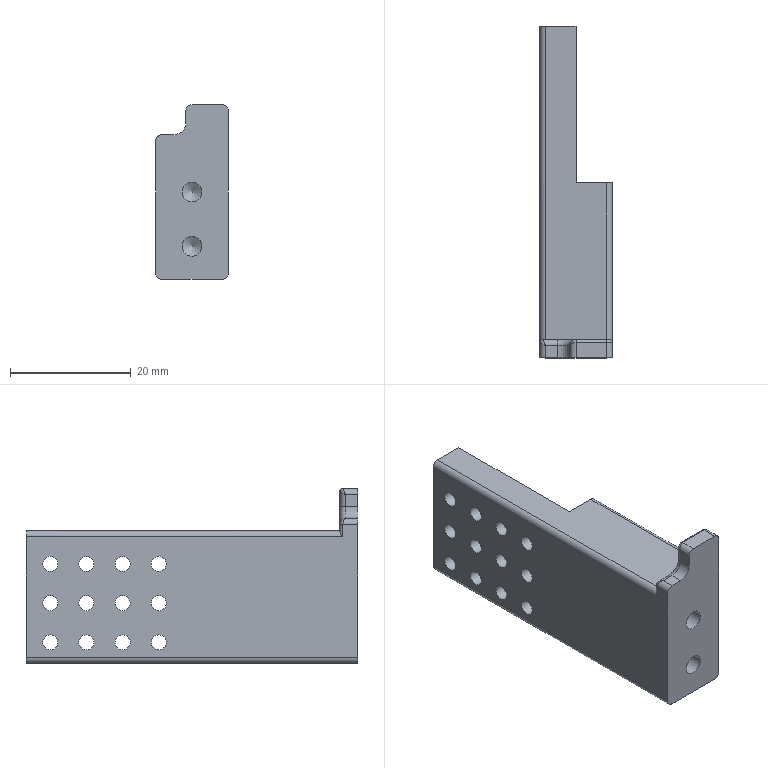Part | 1 solid | 45 faces | box 12 x 55 x 29 mm | volume 10696 mm3 | cylinder 27 | plane 12 | spline 2 | torus 2 | cone 2 | commonest cylinder face diameters 2.5 x12 2 x9 1 x3 3.3 x2 4 x1
STEP:
#1=CARTESIAN_POINT('',(12.,0.,18.));
#2=VERTEX_POINT('',#1);
#3=CARTESIAN_POINT('',(11.,0.,17.));
#4=VERTEX_POINT('',#3);
#5=CARTESIAN_POINT('',(12.,0.,17.));
#6=DIRECTION('',(0.,-1.,0.));
#7=DIRECTION('',(0.,0.,-1.));
#8=AXIS2_PLACEMENT_3D('',#5,#6,#7);
#9=CIRCLE('',#8,1.);
#10=EDGE_CURVE('',#2,#4,#9,.T.);
#11=ORIENTED_EDGE('',*,*,#10,.F.);
#12=CARTESIAN_POINT('',(12.,2.5,18.));
#13=VERTEX_POINT('',#12);
#14=CARTESIAN_POINT('',(12.,0.,18.));
#15=DIRECTION('',(0.,-1.,0.));
#16=VECTOR('',#15,1000.);
#17=LINE('',#14,#16);
#18=EDGE_CURVE('',#13,#2,#17,.T.);
#19=ORIENTED_EDGE('',*,*,#18,.F.);
#20=CARTESIAN_POINT('',(11.,2.,17.));
#21=VERTEX_POINT('',#20);
#22=CARTESIAN_POINT('',(12.,2.,17.));
#23=DIRECTION('',(0.,-0.8944,0.4472));
#24=DIRECTION('',(0.,0.4472,0.8944));
#25=AXIS2_PLACEMENT_3D('',#22,#23,#24);
#26=ELLIPSE('',#25,1.118,1.);
#27=EDGE_CURVE('',#13,#21,#26,.T.);
#28=ORIENTED_EDGE('',*,*,#27,.T.);
#29=CARTESIAN_POINT('',(11.,0.,17.));
#30=DIRECTION('',(0.,1.,0.));
#31=VECTOR('',#30,1000.);
#32=LINE('',#29,#31);
#33=EDGE_CURVE('',#4,#21,#32,.T.);
#34=ORIENTED_EDGE('',*,*,#33,.F.);
#35=EDGE_LOOP('',(#11,#19,#28,#34));
#36=FACE_BOUND('',#35,.T.);
#37=CARTESIAN_POINT('',(12.,0.,17.));
#38=DIRECTION('',(0.,1.,0.));
#39=DIRECTION('',(-1.,0.,0.));
#40=AXIS2_PLACEMENT_3D('',#37,#38,#39);
#41=CYLINDRICAL_SURFACE('',#40,1.);
#42=ADVANCED_FACE('',(#36),#41,.T.);
#43=CARTESIAN_POINT('',(12.,3.,17.5));
#44=VERTEX_POINT('',#43);
#45=CARTESIAN_POINT('',(12.,2.5,17.5));
#46=DIRECTION('',(1.,0.,0.));
#47=DIRECTION('',(0.,1.,0.));
#48=AXIS2_PLACEMENT_3D('',#45,#46,#47);
#49=CIRCLE('',#48,0.5);
#50=EDGE_CURVE('',#44,#13,#49,.T.);
#51=ORIENTED_EDGE('',*,*,#50,.F.);
#52=CARTESIAN_POINT('',(12.,2.,17.));
#53=DIRECTION('',(0.,-0.4472,0.8944));
#54=DIRECTION('',(0.,0.8944,0.4472));
#55=AXIS2_PLACEMENT_3D('',#52,#53,#54);
#56=ELLIPSE('',#55,1.118,1.);
#57=EDGE_CURVE('',#44,#21,#56,.T.);
#58=ORIENTED_EDGE('',*,*,#57,.T.);
#59=ORIENTED_EDGE('',*,*,#27,.F.);
#60=EDGE_LOOP('',(#51,#58,#59));
#61=FACE_BOUND('',#60,.T.);
#62=CARTESIAN_POINT('',(11.,2.,17.));
#63=CARTESIAN_POINT('',(11.,2.,17.));
#64=CARTESIAN_POINT('',(11.,2.,17.));
#65=CARTESIAN_POINT('',(11.,2.131,17.262));
#66=CARTESIAN_POINT('',(11.,2.196,17.196));
#67=CARTESIAN_POINT('',(11.,2.262,17.131));
#68=CARTESIAN_POINT('',(11.217,2.392,17.783));
#69=CARTESIAN_POINT('',(11.101,2.648,17.648));
#70=CARTESIAN_POINT('',(11.217,2.783,17.392));
#71=CARTESIAN_POINT('',(11.738,2.5,18.));
#72=CARTESIAN_POINT('',(11.607,3.,18.));
#73=CARTESIAN_POINT('',(11.738,3.,17.5));
#74=CARTESIAN_POINT('',(12.,2.5,18.));
#75=CARTESIAN_POINT('',(12.,3.,18.));
#76=CARTESIAN_POINT('',(12.,3.,17.5));
#77=(BOUNDED_SURFACE()B_SPLINE_SURFACE(3,2,((#62,#63,#64),(#65,#66,#67),(#68,#69,#70),(#71,#72,#73),(#74,#75,#76)),.UNSPECIFIED.,.F.,.F.,.F.)B_SPLINE_SURFACE_WITH_KNOTS((4,1,4),(3,3),(4.712,5.498,6.283),(0.,1.),.UNSPECIFIED.)GEOMETRIC_REPRESENTATION_ITEM()RATIONAL_B_SPLINE_SURFACE(((1.,1.,1.),(1.,1.,1.),(1.,0.8785,1.),(1.,0.7071,1.),(1.,0.7071,1.)))REPRESENTATION_ITEM('')SURFACE());
#78=ADVANCED_FACE('',(#61),#77,.T.);
#79=CARTESIAN_POINT('',(12.,3.,15.));
#80=VERTEX_POINT('',#79);
#81=CARTESIAN_POINT('',(11.,2.,15.));
#82=VERTEX_POINT('',#81);
#83=CARTESIAN_POINT('',(12.,2.,15.));
#84=DIRECTION('',(0.,0.,1.));
#85=DIRECTION('',(1.,0.,0.));
#86=AXIS2_PLACEMENT_3D('',#83,#84,#85);
#87=CIRCLE('',#86,1.);
#88=EDGE_CURVE('',#80,#82,#87,.T.);
#89=ORIENTED_EDGE('',*,*,#88,.T.);
#90=CARTESIAN_POINT('',(11.,2.,13.));
#91=DIRECTION('',(0.,0.,-1.));
#92=VECTOR('',#91,1000.);
#93=LINE('',#90,#92);
#94=EDGE_CURVE('',#21,#82,#93,.T.);
#95=ORIENTED_EDGE('',*,*,#94,.F.);
#96=ORIENTED_EDGE('',*,*,#57,.F.);
#97=CARTESIAN_POINT('',(12.,3.,18.));
#98=DIRECTION('',(0.,0.,1.));
#99=VECTOR('',#98,1000.);
#100=LINE('',#97,#99);
#101=EDGE_CURVE('',#80,#44,#100,.T.);
#102=ORIENTED_EDGE('',*,*,#101,.F.);
#103=EDGE_LOOP('',(#89,#95,#96,#102));
#104=FACE_BOUND('',#103,.T.);
#105=CARTESIAN_POINT('',(12.,2.,13.));
#106=DIRECTION('',(0.,0.,-1.));
#107=DIRECTION('',(-1.,0.,0.));
#108=AXIS2_PLACEMENT_3D('',#105,#106,#107);
#109=CYLINDRICAL_SURFACE('',#108,1.);
#110=ADVANCED_FACE('',(#104),#109,.T.);
#111=CARTESIAN_POINT('',(9.,3.,12.));
#112=VERTEX_POINT('',#111);
#113=CARTESIAN_POINT('',(9.,2.,13.));
#114=VERTEX_POINT('',#113);
#115=CARTESIAN_POINT('',(9.,2.,12.));
#116=DIRECTION('',(1.,0.,0.));
#117=DIRECTION('',(0.,0.,-1.));
#118=AXIS2_PLACEMENT_3D('',#115,#116,#117);
#119=CIRCLE('',#118,1.);
#120=EDGE_CURVE('',#112,#114,#119,.T.);
#121=ORIENTED_EDGE('',*,*,#120,.T.);
#122=CARTESIAN_POINT('',(9.,2.,15.));
#123=DIRECTION('',(0.,1.,0.));
#124=DIRECTION('',(1.,0.,0.));
#125=AXIS2_PLACEMENT_3D('',#122,#123,#124);
#126=CIRCLE('',#125,2.);
#127=EDGE_CURVE('',#82,#114,#126,.T.);
#128=ORIENTED_EDGE('',*,*,#127,.F.);
#129=ORIENTED_EDGE('',*,*,#88,.F.);
#130=CARTESIAN_POINT('',(9.,3.,15.));
#131=DIRECTION('',(0.,-1.,0.));
#132=DIRECTION('',(1.,0.,0.));
#133=AXIS2_PLACEMENT_3D('',#130,#131,#132);
#134=CIRCLE('',#133,3.);
#135=EDGE_CURVE('',#112,#80,#134,.T.);
#136=ORIENTED_EDGE('',*,*,#135,.F.);
#137=EDGE_LOOP('',(#121,#128,#129,#136));
#138=FACE_BOUND('',#137,.T.);
#139=CARTESIAN_POINT('',(9.,2.,15.));
#140=DIRECTION('',(0.,-1.,0.));
#141=DIRECTION('',(1.,0.,0.));
#142=AXIS2_PLACEMENT_3D('',#139,#140,#141);
#143=TOROIDAL_SURFACE('',#142,3.,1.);
#144=ADVANCED_FACE('',(#138),#143,.T.);
#145=CARTESIAN_POINT('',(6.5,3.,12.));
#146=VERTEX_POINT('',#145);
#147=CARTESIAN_POINT('',(7.,2.,13.));
#148=VERTEX_POINT('',#147);
#149=CARTESIAN_POINT('',(7.,2.,12.));
#150=DIRECTION('',(0.8944,0.4472,0.));
#151=DIRECTION('',(-0.4472,0.8944,0.));
#152=AXIS2_PLACEMENT_3D('',#149,#150,#151);
#153=ELLIPSE('',#152,1.118,1.);
#154=EDGE_CURVE('',#146,#148,#153,.T.);
#155=ORIENTED_EDGE('',*,*,#154,.T.);
#156=CARTESIAN_POINT('',(6.,2.,13.));
#157=DIRECTION('',(-1.,0.,0.));
#158=VECTOR('',#157,1000.);
#159=LINE('',#156,#158);
#160=EDGE_CURVE('',#114,#148,#159,.T.);
#161=ORIENTED_EDGE('',*,*,#160,.F.);
#162=ORIENTED_EDGE('',*,*,#120,.F.);
#163=CARTESIAN_POINT('',(18.,3.,12.));
#164=DIRECTION('',(1.,0.,0.));
#165=VECTOR('',#164,1000.);
#166=LINE('',#163,#165);
#167=EDGE_CURVE('',#146,#112,#166,.T.);
#168=ORIENTED_EDGE('',*,*,#167,.F.);
#169=EDGE_LOOP('',(#155,#161,#162,#168));
#170=FACE_BOUND('',#169,.T.);
#171=CARTESIAN_POINT('',(6.,2.,12.));
#172=DIRECTION('',(-1.,0.,0.));
#173=DIRECTION('',(0.,-1.,0.));
#174=AXIS2_PLACEMENT_3D('',#171,#172,#173);
#175=CYLINDRICAL_SURFACE('',#174,1.);
#176=ADVANCED_FACE('',(#170),#175,.T.);
#177=CARTESIAN_POINT('',(6.,2.5,12.));
#178=VERTEX_POINT('',#177);
#179=CARTESIAN_POINT('',(6.5,2.5,12.));
#180=DIRECTION('',(0.,0.,-1.));
#181=DIRECTION('',(-1.,0.,0.));
#182=AXIS2_PLACEMENT_3D('',#179,#180,#181);
#183=CIRCLE('',#182,0.5);
#184=EDGE_CURVE('',#178,#146,#183,.T.);
#185=ORIENTED_EDGE('',*,*,#184,.F.);
#186=CARTESIAN_POINT('',(7.,2.,12.));
#187=DIRECTION('',(0.4472,0.8944,0.));
#188=DIRECTION('',(-0.8944,0.4472,0.));
#189=AXIS2_PLACEMENT_3D('',#186,#187,#188);
#190=ELLIPSE('',#189,1.118,1.);
#191=EDGE_CURVE('',#178,#148,#190,.T.);
#192=ORIENTED_EDGE('',*,*,#191,.T.);
#193=ORIENTED_EDGE('',*,*,#154,.F.);
#194=EDGE_LOOP('',(#185,#192,#193));
#195=FACE_BOUND('',#194,.T.);
#196=CARTESIAN_POINT('',(7.,2.,13.));
#197=CARTESIAN_POINT('',(7.,2.,13.));
#198=CARTESIAN_POINT('',(7.,2.,13.));
#199=CARTESIAN_POINT('',(6.869,2.262,13.));
#200=CARTESIAN_POINT('',(6.804,2.196,13.));
#201=CARTESIAN_POINT('',(6.738,2.131,13.));
#202=CARTESIAN_POINT('',(6.608,2.783,12.783));
#203=CARTESIAN_POINT('',(6.352,2.648,12.899));
#204=CARTESIAN_POINT('',(6.217,2.392,12.783));
#205=CARTESIAN_POINT('',(6.5,3.,12.262));
#206=CARTESIAN_POINT('',(6.,3.,12.393));
#207=CARTESIAN_POINT('',(6.,2.5,12.262));
#208=CARTESIAN_POINT('',(6.5,3.,12.));
#209=CARTESIAN_POINT('',(6.,3.,12.));
#210=CARTESIAN_POINT('',(6.,2.5,12.));
#211=(BOUNDED_SURFACE()B_SPLINE_SURFACE(3,2,((#196,#197,#198),(#199,#200,#201),(#202,#203,#204),(#205,#206,#207),(#208,#209,#210)),.UNSPECIFIED.,.F.,.F.,.F.)B_SPLINE_SURFACE_WITH_KNOTS((4,1,4),(3,3),(4.712,5.498,6.283),(0.,1.),.UNSPECIFIED.)GEOMETRIC_REPRESENTATION_ITEM()RATIONAL_B_SPLINE_SURFACE(((1.,1.,1.),(1.,1.,1.),(1.,0.8785,1.),(1.,0.7071,1.),(1.,0.7071,1.)))REPRESENTATION_ITEM('')SURFACE());
#212=ADVANCED_FACE('',(#195),#211,.T.);
#213=CARTESIAN_POINT('',(7.,0.,13.));
#214=VERTEX_POINT('',#213);
#215=CARTESIAN_POINT('',(6.,0.,12.));
#216=VERTEX_POINT('',#215);
#217=CARTESIAN_POINT('',(7.,0.,12.));
#218=DIRECTION('',(0.,-1.,0.));
#219=DIRECTION('',(0.,0.,-1.));
#220=AXIS2_PLACEMENT_3D('',#217,#218,#219);
#221=CIRCLE('',#220,1.);
#222=EDGE_CURVE('',#214,#216,#221,.T.);
#223=ORIENTED_EDGE('',*,*,#222,.F.);
#224=CARTESIAN_POINT('',(7.,0.,13.));
#225=DIRECTION('',(0.,-1.,0.));
#226=VECTOR('',#225,1000.);
#227=LINE('',#224,#226);
#228=EDGE_CURVE('',#148,#214,#227,.T.);
#229=ORIENTED_EDGE('',*,*,#228,.F.);
#230=ORIENTED_EDGE('',*,*,#191,.F.);
#231=CARTESIAN_POINT('',(6.,55.,12.));
#232=DIRECTION('',(0.,1.,0.));
#233=VECTOR('',#232,1000.);
#234=LINE('',#231,#233);
#235=EDGE_CURVE('',#216,#178,#234,.T.);
#236=ORIENTED_EDGE('',*,*,#235,.F.);
#237=EDGE_LOOP('',(#223,#229,#230,#236));
#238=FACE_BOUND('',#237,.T.);
#239=CARTESIAN_POINT('',(7.,55.,12.));
#240=DIRECTION('',(0.,1.,0.));
#241=DIRECTION('',(0.,0.,1.));
#242=AXIS2_PLACEMENT_3D('',#239,#240,#241);
#243=CYLINDRICAL_SURFACE('',#242,1.);
#244=ADVANCED_FACE('',(#238),#243,.T.);
#245=CARTESIAN_POINT('',(11.,0.,15.));
#246=VERTEX_POINT('',#245);
#247=CARTESIAN_POINT('',(11.,0.,15.));
#248=DIRECTION('',(0.,-1.,0.));
#249=VECTOR('',#248,1000.);
#250=LINE('',#247,#249);
#251=EDGE_CURVE('',#82,#246,#250,.T.);
#252=ORIENTED_EDGE('',*,*,#251,.F.);
#253=ORIENTED_EDGE('',*,*,#127,.T.);
#254=CARTESIAN_POINT('',(9.,0.,13.));
#255=VERTEX_POINT('',#254);
#256=CARTESIAN_POINT('',(9.,3.,13.));
#257=DIRECTION('',(0.,1.,0.));
#258=VECTOR('',#257,1000.);
#259=LINE('',#256,#258);
#260=EDGE_CURVE('',#255,#114,#259,.T.);
#261=ORIENTED_EDGE('',*,*,#260,.F.);
#262=CARTESIAN_POINT('',(9.,0.,15.));
#263=DIRECTION('',(0.,1.,0.));
#264=DIRECTION('',(0.,0.,-1.));
#265=AXIS2_PLACEMENT_3D('',#262,#263,#264);
#266=CIRCLE('',#265,2.);
#267=EDGE_CURVE('',#246,#255,#266,.T.);
#268=ORIENTED_EDGE('',*,*,#267,.F.);
#269=EDGE_LOOP('',(#252,#253,#261,#268));
#270=FACE_BOUND('',#269,.T.);
#271=CARTESIAN_POINT('',(9.,0.,15.));
#272=DIRECTION('',(0.,-1.,0.));
#273=DIRECTION('',(1.,0.,0.));
#274=AXIS2_PLACEMENT_3D('',#271,#272,#273);
#275=CYLINDRICAL_SURFACE('',#274,2.);
#276=ADVANCED_FACE('',(#270),#275,.F.);
#277=CARTESIAN_POINT('',(11.,0.,13.));
#278=DIRECTION('',(0.,0.,-1.));
#279=VECTOR('',#278,1000.);
#280=LINE('',#277,#279);
#281=EDGE_CURVE('',#4,#246,#280,.T.);
#282=ORIENTED_EDGE('',*,*,#281,.F.);
#283=ORIENTED_EDGE('',*,*,#33,.T.);
#284=ORIENTED_EDGE('',*,*,#94,.T.);
#285=ORIENTED_EDGE('',*,*,#251,.T.);
#286=EDGE_LOOP('',(#282,#283,#284,#285));
#287=FACE_BOUND('',#286,.T.);
#288=CARTESIAN_POINT('',(11.,0.,13.));
#289=DIRECTION('',(1.,0.,0.));
#290=DIRECTION('',(0.,1.,0.));
#291=AXIS2_PLACEMENT_3D('',#288,#289,#290);
#292=PLANE('',#291);
#293=ADVANCED_FACE('',(#287),#292,.F.);
#294=ORIENTED_EDGE('',*,*,#260,.T.);
#295=ORIENTED_EDGE('',*,*,#160,.T.);
#296=ORIENTED_EDGE('',*,*,#228,.T.);
#297=CARTESIAN_POINT('',(6.,0.,13.));
#298=DIRECTION('',(-1.,0.,0.));
#299=VECTOR('',#298,1000.);
#300=LINE('',#297,#299);
#301=EDGE_CURVE('',#255,#214,#300,.T.);
#302=ORIENTED_EDGE('',*,*,#301,.F.);
#303=EDGE_LOOP('',(#294,#295,#296,#302));
#304=FACE_BOUND('',#303,.T.);
#305=CARTESIAN_POINT('',(6.,0.,13.));
#306=DIRECTION('',(0.,0.,-1.));
#307=DIRECTION('',(-1.,0.,0.));
#308=AXIS2_PLACEMENT_3D('',#305,#306,#307);
#309=PLANE('',#308);
#310=ADVANCED_FACE('',(#304),#309,.F.);
#311=CARTESIAN_POINT('',(6.,2.5,10.));
#312=VERTEX_POINT('',#311);
#313=CARTESIAN_POINT('',(6.,2.5,11.));
#314=DIRECTION('',(0.,0.,1.));
#315=VECTOR('',#314,1000.);
#316=LINE('',#313,#315);
#317=EDGE_CURVE('',#312,#178,#316,.T.);
#318=ORIENTED_EDGE('',*,*,#317,.T.);
#319=ORIENTED_EDGE('',*,*,#184,.T.);
#320=CARTESIAN_POINT('',(6.5,3.,10.866));
#321=VERTEX_POINT('',#320);
#322=CARTESIAN_POINT('',(6.5,3.,18.));
#323=DIRECTION('',(0.,0.,-1.));
#324=VECTOR('',#323,1000.);
#325=LINE('',#322,#324);
#326=EDGE_CURVE('',#146,#321,#325,.T.);
#327=ORIENTED_EDGE('',*,*,#326,.T.);
#328=CARTESIAN_POINT('',(6.5,3.,10.866));
#329=CARTESIAN_POINT('',(6.155,3.,10.667));
#330=CARTESIAN_POINT('',(6.,2.725,10.319));
#331=CARTESIAN_POINT('',(6.,2.5,10.));
#332=B_SPLINE_CURVE_WITH_KNOTS('',3,(#328,#329,#330,#331),.UNSPECIFIED.,.F.,.F.,(4,4),(0.,0.001171),.UNSPECIFIED.);
#333=EDGE_CURVE('',#321,#312,#332,.T.);
#334=ORIENTED_EDGE('',*,*,#333,.T.);
#335=EDGE_LOOP('',(#318,#319,#327,#334));
#336=FACE_BOUND('',#335,.T.);
#337=CARTESIAN_POINT('',(6.5,2.5,18.));
#338=DIRECTION('',(0.,0.,-1.));
#339=DIRECTION('',(1.,0.,0.));
#340=AXIS2_PLACEMENT_3D('',#337,#338,#339);
#341=CYLINDRICAL_SURFACE('',#340,0.5);
#342=ADVANCED_FACE('',(#336),#341,.T.);
#343=CARTESIAN_POINT('',(17.,3.,17.5));
#344=VERTEX_POINT('',#343);
#345=CARTESIAN_POINT('',(18.,3.,17.5));
#346=DIRECTION('',(-1.,0.,0.));
#347=VECTOR('',#346,1000.);
#348=LINE('',#345,#347);
#349=EDGE_CURVE('',#344,#44,#348,.T.);
#350=ORIENTED_EDGE('',*,*,#349,.T.);
#351=ORIENTED_EDGE('',*,*,#50,.T.);
#352=CARTESIAN_POINT('',(17.,2.5,18.));
#353=VERTEX_POINT('',#352);
#354=CARTESIAN_POINT('',(12.,2.5,18.));
#355=DIRECTION('',(1.,0.,0.));
#356=VECTOR('',#355,1000.);
#357=LINE('',#354,#356);
#358=EDGE_CURVE('',#13,#353,#357,.T.);
#359=ORIENTED_EDGE('',*,*,#358,.T.);
#360=CARTESIAN_POINT('',(17.,2.5,17.5));
#361=DIRECTION('',(1.,0.,0.));
#362=DIRECTION('',(0.,0.,-1.));
#363=AXIS2_PLACEMENT_3D('',#360,#361,#362);
#364=CIRCLE('',#363,0.5);
#365=EDGE_CURVE('',#344,#353,#364,.T.);
#366=ORIENTED_EDGE('',*,*,#365,.F.);
#367=EDGE_LOOP('',(#350,#351,#359,#366));
#368=FACE_BOUND('',#367,.T.);
#369=CARTESIAN_POINT('',(12.,2.5,17.5));
#370=DIRECTION('',(1.,0.,0.));
#371=DIRECTION('',(0.,-1.,0.));
#372=AXIS2_PLACEMENT_3D('',#369,#370,#371);
#373=CYLINDRICAL_SURFACE('',#372,0.5);
#374=ADVANCED_FACE('',(#368),#373,.T.);
#375=CARTESIAN_POINT('',(17.5,3.,17.));
#376=VERTEX_POINT('',#375);
#377=CARTESIAN_POINT('',(18.,2.5,17.));
#378=VERTEX_POINT('',#377);
#379=CARTESIAN_POINT('',(17.5,2.5,17.));
#380=DIRECTION('',(0.,0.,-1.));
#381=DIRECTION('',(-1.,0.,0.));
#382=AXIS2_PLACEMENT_3D('',#379,#380,#381);
#383=CIRCLE('',#382,0.5);
#384=EDGE_CURVE('',#376,#378,#383,.T.);
#385=ORIENTED_EDGE('',*,*,#384,.F.);
#386=CARTESIAN_POINT('',(17.,3.,17.));
#387=DIRECTION('',(0.,-1.,0.));
#388=DIRECTION('',(-1.,0.,0.));
#389=AXIS2_PLACEMENT_3D('',#386,#387,#388);
#390=CIRCLE('',#389,0.5);
#391=EDGE_CURVE('',#376,#344,#390,.T.);
#392=ORIENTED_EDGE('',*,*,#391,.T.);
#393=ORIENTED_EDGE('',*,*,#365,.T.);
#394=CARTESIAN_POINT('',(17.,2.5,17.));
#395=DIRECTION('',(0.,1.,0.));
#396=DIRECTION('',(-1.,0.,0.));
#397=AXIS2_PLACEMENT_3D('',#394,#395,#396);
#398=CIRCLE('',#397,1.);
#399=EDGE_CURVE('',#353,#378,#398,.T.);
#400=ORIENTED_EDGE('',*,*,#399,.T.);
#401=EDGE_LOOP('',(#385,#392,#393,#400));
#402=FACE_BOUND('',#401,.T.);
#403=CARTESIAN_POINT('',(17.,2.5,17.));
#404=DIRECTION('',(0.,-1.,0.));
#405=DIRECTION('',(-1.,0.,0.));
#406=AXIS2_PLACEMENT_3D('',#403,#404,#405);
#407=TOROIDAL_SURFACE('',#406,0.5,0.5);
#408=ADVANCED_FACE('',(#402),#407,.T.);
#409=CARTESIAN_POINT('',(18.,2.5,10.));
#410=VERTEX_POINT('',#409);
#411=CARTESIAN_POINT('',(17.5,3.,10.866));
#412=VERTEX_POINT('',#411);
#413=CARTESIAN_POINT('',(17.5,3.,10.866));
#414=CARTESIAN_POINT('',(17.845,3.,10.667));
#415=CARTESIAN_POINT('',(18.,2.725,10.319));
#416=CARTESIAN_POINT('',(18.,2.5,10.));
#417=B_SPLINE_CURVE_WITH_KNOTS('',3,(#413,#414,#415,#416),.UNSPECIFIED.,.F.,.F.,(4,4),(0.,0.001171),.UNSPECIFIED.);
#418=EDGE_CURVE('',#410,#412,#417,.F.);
#419=ORIENTED_EDGE('',*,*,#418,.T.);
#420=CARTESIAN_POINT('',(17.5,3.,18.));
#421=DIRECTION('',(0.,0.,1.));
#422=VECTOR('',#421,1000.);
#423=LINE('',#420,#422);
#424=EDGE_CURVE('',#412,#376,#423,.T.);
#425=ORIENTED_EDGE('',*,*,#424,.T.);
#426=ORIENTED_EDGE('',*,*,#384,.T.);
#427=CARTESIAN_POINT('',(18.,2.5,11.));
#428=DIRECTION('',(0.,0.,-1.));
#429=VECTOR('',#428,1000.);
#430=LINE('',#427,#429);
#431=EDGE_CURVE('',#378,#410,#430,.T.);
#432=ORIENTED_EDGE('',*,*,#431,.T.);
#433=EDGE_LOOP('',(#419,#425,#426,#432));
#434=FACE_BOUND('',#433,.T.);
#435=CARTESIAN_POINT('',(17.5,2.5,11.));
#436=DIRECTION('',(0.,0.,-1.));
#437=DIRECTION('',(1.,0.,0.));
#438=AXIS2_PLACEMENT_3D('',#435,#436,#437);
#439=CYLINDRICAL_SURFACE('',#438,0.5);
#440=ADVANCED_FACE('',(#434),#439,.T.);
#441=CARTESIAN_POINT('',(17.,0.,18.));
#442=VERTEX_POINT('',#441);
#443=CARTESIAN_POINT('',(17.,0.,18.));
#444=DIRECTION('',(0.,-1.,0.));
#445=VECTOR('',#444,1000.);
#446=LINE('',#443,#445);
#447=EDGE_CURVE('',#353,#442,#446,.T.);
#448=ORIENTED_EDGE('',*,*,#447,.T.);
#449=CARTESIAN_POINT('',(18.,0.,17.));
#450=VERTEX_POINT('',#449);
#451=CARTESIAN_POINT('',(17.,0.,17.));
#452=DIRECTION('',(0.,1.,0.));
#453=DIRECTION('',(0.,0.,-1.));
#454=AXIS2_PLACEMENT_3D('',#451,#452,#453);
#455=CIRCLE('',#454,1.);
#456=EDGE_CURVE('',#442,#450,#455,.T.);
#457=ORIENTED_EDGE('',*,*,#456,.T.);
#458=CARTESIAN_POINT('',(18.,55.,17.));
#459=DIRECTION('',(0.,1.,0.));
#460=VECTOR('',#459,1000.);
#461=LINE('',#458,#460);
#462=EDGE_CURVE('',#450,#378,#461,.T.);
#463=ORIENTED_EDGE('',*,*,#462,.T.);
#464=ORIENTED_EDGE('',*,*,#399,.F.);
#465=EDGE_LOOP('',(#448,#457,#463,#464));
#466=FACE_BOUND('',#465,.T.);
#467=CARTESIAN_POINT('',(17.,0.,17.));
#468=DIRECTION('',(0.,-1.,0.));
#469=DIRECTION('',(0.,0.,-1.));
#470=AXIS2_PLACEMENT_3D('',#467,#468,#469);
#471=CYLINDRICAL_SURFACE('',#470,1.);
#472=ADVANCED_FACE('',(#466),#471,.T.);
#473=CARTESIAN_POINT('',(18.,29.,10.));
#474=VERTEX_POINT('',#473);
#475=CARTESIAN_POINT('',(17.,29.,11.));
#476=VERTEX_POINT('',#475);
#477=CARTESIAN_POINT('',(17.,29.,10.));
#478=DIRECTION('',(0.,-1.,0.));
#479=DIRECTION('',(0.,0.,-1.));
#480=AXIS2_PLACEMENT_3D('',#477,#478,#479);
#481=CIRCLE('',#480,1.);
#482=EDGE_CURVE('',#474,#476,#481,.T.);
#483=ORIENTED_EDGE('',*,*,#482,.T.);
#484=CARTESIAN_POINT('',(17.,3.,11.));
#485=VERTEX_POINT('',#484);
#486=CARTESIAN_POINT('',(17.,55.,11.));
#487=DIRECTION('',(0.,-1.,0.));
#488=VECTOR('',#487,1000.);
#489=LINE('',#486,#488);
#490=EDGE_CURVE('',#476,#485,#489,.T.);
#491=ORIENTED_EDGE('',*,*,#490,.T.);
#492=CARTESIAN_POINT('',(17.,3.,10.));
#493=DIRECTION('',(0.,1.,0.));
#494=DIRECTION('',(-1.,0.,0.));
#495=AXIS2_PLACEMENT_3D('',#492,#493,#494);
#496=CIRCLE('',#495,1.);
#497=EDGE_CURVE('',#485,#412,#496,.T.);
#498=ORIENTED_EDGE('',*,*,#497,.T.);
#499=ORIENTED_EDGE('',*,*,#418,.F.);
#500=CARTESIAN_POINT('',(18.,55.,10.));
#501=DIRECTION('',(0.,1.,0.));
#502=VECTOR('',#501,1000.);
#503=LINE('',#500,#502);
#504=EDGE_CURVE('',#410,#474,#503,.T.);
#505=ORIENTED_EDGE('',*,*,#504,.T.);
#506=EDGE_LOOP('',(#483,#491,#498,#499,#505));
#507=FACE_BOUND('',#506,.T.);
#508=CARTESIAN_POINT('',(17.,55.,10.));
#509=DIRECTION('',(0.,-1.,0.));
#510=DIRECTION('',(0.,0.,-1.));
#511=AXIS2_PLACEMENT_3D('',#508,#509,#510);
#512=CYLINDRICAL_SURFACE('',#511,1.);
#513=ADVANCED_FACE('',(#507),#512,.T.);
#514=CARTESIAN_POINT('',(7.,55.,11.));
#515=VERTEX_POINT('',#514);
#516=CARTESIAN_POINT('',(6.,55.,10.));
#517=VERTEX_POINT('',#516);
#518=CARTESIAN_POINT('',(7.,55.,10.));
#519=DIRECTION('',(0.,-1.,0.));
#520=DIRECTION('',(0.,0.,-1.));
#521=AXIS2_PLACEMENT_3D('',#518,#519,#520);
#522=CIRCLE('',#521,1.);
#523=EDGE_CURVE('',#515,#517,#522,.T.);
#524=ORIENTED_EDGE('',*,*,#523,.T.);
#525=CARTESIAN_POINT('',(6.,55.,10.));
#526=DIRECTION('',(0.,-1.,0.));
#527=VECTOR('',#526,1000.);
#528=LINE('',#525,#527);
#529=EDGE_CURVE('',#517,#312,#528,.T.);
#530=ORIENTED_EDGE('',*,*,#529,.T.);
#531=ORIENTED_EDGE('',*,*,#333,.F.);
#532=CARTESIAN_POINT('',(7.,3.,11.));
#533=VERTEX_POINT('',#532);
#534=CARTESIAN_POINT('',(7.,3.,10.));
#535=DIRECTION('',(0.,1.,0.));
#536=DIRECTION('',(-1.,0.,0.));
#537=AXIS2_PLACEMENT_3D('',#534,#535,#536);
#538=CIRCLE('',#537,1.);
#539=EDGE_CURVE('',#321,#533,#538,.T.);
#540=ORIENTED_EDGE('',*,*,#539,.T.);
#541=CARTESIAN_POINT('',(7.,55.,11.));
#542=DIRECTION('',(0.,1.,0.));
#543=VECTOR('',#542,1000.);
#544=LINE('',#541,#543);
#545=EDGE_CURVE('',#533,#515,#544,.T.);
#546=ORIENTED_EDGE('',*,*,#545,.T.);
#547=EDGE_LOOP('',(#524,#530,#531,#540,#546));
#548=FACE_BOUND('',#547,.T.);
#549=CARTESIAN_POINT('',(7.,55.,10.));
#550=DIRECTION('',(0.,-1.,0.));
#551=DIRECTION('',(0.,0.,-1.));
#552=AXIS2_PLACEMENT_3D('',#549,#550,#551);
#553=CYLINDRICAL_SURFACE('',#552,1.);
#554=ADVANCED_FACE('',(#548),#553,.T.);
#555=CARTESIAN_POINT('',(17.,29.,-11.));
#556=VERTEX_POINT('',#555);
#557=CARTESIAN_POINT('',(18.,29.,-10.));
#558=VERTEX_POINT('',#557);
#559=CARTESIAN_POINT('',(17.,29.,-10.));
#560=DIRECTION('',(0.,-1.,0.));
#561=DIRECTION('',(0.,0.,-1.));
#562=AXIS2_PLACEMENT_3D('',#559,#560,#561);
#563=CIRCLE('',#562,1.);
#564=EDGE_CURVE('',#556,#558,#563,.T.);
#565=ORIENTED_EDGE('',*,*,#564,.T.);
#566=CARTESIAN_POINT('',(18.,0.,-10.));
#567=VERTEX_POINT('',#566);
#568=CARTESIAN_POINT('',(18.,55.,-10.));
#569=DIRECTION('',(0.,-1.,0.));
#570=VECTOR('',#569,1000.);
#571=LINE('',#568,#570);
#572=EDGE_CURVE('',#558,#567,#571,.T.);
#573=ORIENTED_EDGE('',*,*,#572,.T.);
#574=CARTESIAN_POINT('',(17.,0.,-11.));
#575=VERTEX_POINT('',#574);
#576=CARTESIAN_POINT('',(17.,0.,-10.));
#577=DIRECTION('',(0.,1.,0.));
#578=DIRECTION('',(0.,0.,-1.));
#579=AXIS2_PLACEMENT_3D('',#576,#577,#578);
#580=CIRCLE('',#579,1.);
#581=EDGE_CURVE('',#567,#575,#580,.T.);
#582=ORIENTED_EDGE('',*,*,#581,.T.);
#583=CARTESIAN_POINT('',(17.,55.,-11.));
#584=DIRECTION('',(0.,1.,0.));
#585=VECTOR('',#584,1000.);
#586=LINE('',#583,#585);
#587=EDGE_CURVE('',#575,#556,#586,.T.);
#588=ORIENTED_EDGE('',*,*,#587,.T.);
#589=EDGE_LOOP('',(#565,#573,#582,#588));
#590=FACE_BOUND('',#589,.T.);
#591=CARTESIAN_POINT('',(17.,55.,-10.));
#592=DIRECTION('',(0.,-1.,0.));
#593=DIRECTION('',(0.,0.,-1.));
#594=AXIS2_PLACEMENT_3D('',#591,#592,#593);
#595=CYLINDRICAL_SURFACE('',#594,1.);
#596=ADVANCED_FACE('',(#590),#595,.T.);
#597=CARTESIAN_POINT('',(6.,55.,-10.));
#598=VERTEX_POINT('',#597);
#599=CARTESIAN_POINT('',(7.,55.,-11.));
#600=VERTEX_POINT('',#599);
#601=CARTESIAN_POINT('',(7.,55.,-10.));
#602=DIRECTION('',(0.,-1.,0.));
#603=DIRECTION('',(0.,0.,-1.));
#604=AXIS2_PLACEMENT_3D('',#601,#602,#603);
#605=CIRCLE('',#604,1.);
#606=EDGE_CURVE('',#598,#600,#605,.T.);
#607=ORIENTED_EDGE('',*,*,#606,.T.);
#608=CARTESIAN_POINT('',(7.,0.,-11.));
#609=VERTEX_POINT('',#608);
#610=CARTESIAN_POINT('',(7.,55.,-11.));
#611=DIRECTION('',(0.,-1.,0.));
#612=VECTOR('',#611,1000.);
#613=LINE('',#610,#612);
#614=EDGE_CURVE('',#600,#609,#613,.T.);
#615=ORIENTED_EDGE('',*,*,#614,.T.);
#616=CARTESIAN_POINT('',(6.,0.,-10.));
#617=VERTEX_POINT('',#616);
#618=CARTESIAN_POINT('',(7.,0.,-10.));
#619=DIRECTION('',(0.,1.,0.));
#620=DIRECTION('',(0.,0.,-1.));
#621=AXIS2_PLACEMENT_3D('',#618,#619,#620);
#622=CIRCLE('',#621,1.);
#623=EDGE_CURVE('',#609,#617,#622,.T.);
#624=ORIENTED_EDGE('',*,*,#623,.T.);
#625=CARTESIAN_POINT('',(6.,55.,-10.));
#626=DIRECTION('',(0.,1.,0.));
#627=VECTOR('',#626,1000.);
#628=LINE('',#625,#627);
#629=EDGE_CURVE('',#617,#598,#628,.T.);
#630=ORIENTED_EDGE('',*,*,#629,.T.);
#631=EDGE_LOOP('',(#607,#615,#624,#630));
#632=FACE_BOUND('',#631,.T.);
#633=CARTESIAN_POINT('',(7.,55.,-10.));
#634=DIRECTION('',(0.,-1.,0.));
#635=DIRECTION('',(0.,0.,-1.));
#636=AXIS2_PLACEMENT_3D('',#633,#634,#635);
#637=CYLINDRICAL_SURFACE('',#636,1.);
#638=ADVANCED_FACE('',(#632),#637,.T.);
#639=ORIENTED_EDGE('',*,*,#358,.F.);
#640=ORIENTED_EDGE('',*,*,#18,.T.);
#641=CARTESIAN_POINT('',(18.,0.,18.));
#642=DIRECTION('',(-1.,0.,0.));
#643=VECTOR('',#642,1000.);
#644=LINE('',#641,#643);
#645=EDGE_CURVE('',#442,#2,#644,.T.);
#646=ORIENTED_EDGE('',*,*,#645,.F.);
#647=ORIENTED_EDGE('',*,*,#447,.F.);
#648=EDGE_LOOP('',(#639,#640,#646,#647));
#649=FACE_BOUND('',#648,.T.);
#650=CARTESIAN_POINT('',(12.,0.,18.));
#651=DIRECTION('',(0.,0.,-1.));
#652=DIRECTION('',(1.,0.,0.));
#653=AXIS2_PLACEMENT_3D('',#650,#651,#652);
#654=PLANE('',#653);
#655=ADVANCED_FACE('',(#649),#654,.F.);
#656=ORIENTED_EDGE('',*,*,#135,.T.);
#657=ORIENTED_EDGE('',*,*,#101,.T.);
#658=ORIENTED_EDGE('',*,*,#349,.F.);
#659=ORIENTED_EDGE('',*,*,#391,.F.);
#660=ORIENTED_EDGE('',*,*,#424,.F.);
#661=ORIENTED_EDGE('',*,*,#497,.F.);
#662=CARTESIAN_POINT('',(18.,3.,11.));
#663=DIRECTION('',(1.,0.,0.));
#664=VECTOR('',#663,1000.);
#665=LINE('',#662,#664);
#666=EDGE_CURVE('',#533,#485,#665,.T.);
#667=ORIENTED_EDGE('',*,*,#666,.F.);
#668=ORIENTED_EDGE('',*,*,#539,.F.);
#669=ORIENTED_EDGE('',*,*,#326,.F.);
#670=ORIENTED_EDGE('',*,*,#167,.T.);
#671=EDGE_LOOP('',(#656,#657,#658,#659,#660,#661,#667,#668,#669,#670));
#672=FACE_BOUND('',#671,.T.);
#673=CARTESIAN_POINT('',(18.,3.,18.));
#674=DIRECTION('',(0.,-1.,0.));
#675=DIRECTION('',(-1.,0.,0.));
#676=AXIS2_PLACEMENT_3D('',#673,#674,#675);
#677=PLANE('',#676);
#678=ADVANCED_FACE('',(#672),#677,.F.);
#679=CARTESIAN_POINT('',(12.,29.,11.));
#680=VERTEX_POINT('',#679);
#681=CARTESIAN_POINT('',(12.,55.,11.));
#682=VERTEX_POINT('',#681);
#683=CARTESIAN_POINT('',(12.,55.,11.));
#684=DIRECTION('',(0.,1.,0.));
#685=VECTOR('',#684,1000.);
#686=LINE('',#683,#685);
#687=EDGE_CURVE('',#680,#682,#686,.T.);
#688=ORIENTED_EDGE('',*,*,#687,.F.);
#689=CARTESIAN_POINT('',(12.,29.,-11.));
#690=VERTEX_POINT('',#689);
#691=CARTESIAN_POINT('',(12.,29.,-11.));
#692=DIRECTION('',(0.,0.,1.));
#693=VECTOR('',#692,1000.);
#694=LINE('',#691,#693);
#695=EDGE_CURVE('',#690,#680,#694,.T.);
#696=ORIENTED_EDGE('',*,*,#695,.F.);
#697=CARTESIAN_POINT('',(12.,55.,-11.));
#698=VERTEX_POINT('',#697);
#699=CARTESIAN_POINT('',(12.,55.,-11.));
#700=DIRECTION('',(0.,-1.,0.));
#701=VECTOR('',#700,1000.);
#702=LINE('',#699,#701);
#703=EDGE_CURVE('',#698,#690,#702,.T.);
#704=ORIENTED_EDGE('',*,*,#703,.F.);
#705=CARTESIAN_POINT('',(12.,55.,0.));
#706=DIRECTION('',(0.,0.,-1.));
#707=VECTOR('',#706,1000.);
#708=LINE('',#705,#707);
#709=EDGE_CURVE('',#682,#698,#708,.T.);
#710=ORIENTED_EDGE('',*,*,#709,.F.);
#711=EDGE_LOOP('',(#688,#696,#704,#710));
#712=FACE_BOUND('',#711,.T.);
#713=CARTESIAN_POINT('',(12.,33.,6.75));
#714=VERTEX_POINT('',#713);
#715=CARTESIAN_POINT('',(12.,33.,5.5));
#716=DIRECTION('',(-1.,0.,0.));
#717=DIRECTION('',(0.,0.,1.));
#718=AXIS2_PLACEMENT_3D('',#715,#716,#717);
#719=CIRCLE('',#718,1.25);
#720=EDGE_CURVE('',#714,#714,#719,.T.);
#721=ORIENTED_EDGE('',*,*,#720,.T.);
#722=EDGE_LOOP('',(#721));
#723=FACE_BOUND('',#722,.T.);
#724=CARTESIAN_POINT('',(12.,33.,0.25));
#725=VERTEX_POINT('',#724);
#726=CARTESIAN_POINT('',(12.,33.,-1.));
#727=DIRECTION('',(-1.,0.,0.));
#728=DIRECTION('',(0.,0.,1.));
#729=AXIS2_PLACEMENT_3D('',#726,#727,#728);
#730=CIRCLE('',#729,1.25);
#731=EDGE_CURVE('',#725,#725,#730,.T.);
#732=ORIENTED_EDGE('',*,*,#731,.T.);
#733=EDGE_LOOP('',(#732));
#734=FACE_BOUND('',#733,.T.);
#735=CARTESIAN_POINT('',(12.,33.,-6.25));
#736=VERTEX_POINT('',#735);
#737=CARTESIAN_POINT('',(12.,33.,-7.5));
#738=DIRECTION('',(-1.,0.,0.));
#739=DIRECTION('',(0.,0.,1.));
#740=AXIS2_PLACEMENT_3D('',#737,#738,#739);
#741=CIRCLE('',#740,1.25);
#742=EDGE_CURVE('',#736,#736,#741,.T.);
#743=ORIENTED_EDGE('',*,*,#742,.T.);
#744=EDGE_LOOP('',(#743));
#745=FACE_BOUND('',#744,.T.);
#746=CARTESIAN_POINT('',(12.,39.,-6.25));
#747=VERTEX_POINT('',#746);
#748=CARTESIAN_POINT('',(12.,39.,-7.5));
#749=DIRECTION('',(-1.,0.,0.));
#750=DIRECTION('',(0.,0.,1.));
#751=AXIS2_PLACEMENT_3D('',#748,#749,#750);
#752=CIRCLE('',#751,1.25);
#753=EDGE_CURVE('',#747,#747,#752,.T.);
#754=ORIENTED_EDGE('',*,*,#753,.T.);
#755=EDGE_LOOP('',(#754));
#756=FACE_BOUND('',#755,.T.);
#757=CARTESIAN_POINT('',(12.,39.,0.25));
#758=VERTEX_POINT('',#757);
#759=CARTESIAN_POINT('',(12.,39.,-1.));
#760=DIRECTION('',(-1.,0.,0.));
#761=DIRECTION('',(0.,0.,1.));
#762=AXIS2_PLACEMENT_3D('',#759,#760,#761);
#763=CIRCLE('',#762,1.25);
#764=EDGE_CURVE('',#758,#758,#763,.T.);
#765=ORIENTED_EDGE('',*,*,#764,.T.);
#766=EDGE_LOOP('',(#765));
#767=FACE_BOUND('',#766,.T.);
#768=CARTESIAN_POINT('',(12.,39.,6.75));
#769=VERTEX_POINT('',#768);
#770=CARTESIAN_POINT('',(12.,39.,5.5));
#771=DIRECTION('',(-1.,0.,0.));
#772=DIRECTION('',(0.,0.,1.));
#773=AXIS2_PLACEMENT_3D('',#770,#771,#772);
#774=CIRCLE('',#773,1.25);
#775=EDGE_CURVE('',#769,#769,#774,.T.);
#776=ORIENTED_EDGE('',*,*,#775,.T.);
#777=EDGE_LOOP('',(#776));
#778=FACE_BOUND('',#777,.T.);
#779=CARTESIAN_POINT('',(12.,45.,6.75));
#780=VERTEX_POINT('',#779);
#781=CARTESIAN_POINT('',(12.,45.,5.5));
#782=DIRECTION('',(-1.,0.,0.));
#783=DIRECTION('',(0.,0.,1.));
#784=AXIS2_PLACEMENT_3D('',#781,#782,#783);
#785=CIRCLE('',#784,1.25);
#786=EDGE_CURVE('',#780,#780,#785,.T.);
#787=ORIENTED_EDGE('',*,*,#786,.T.);
#788=EDGE_LOOP('',(#787));
#789=FACE_BOUND('',#788,.T.);
#790=CARTESIAN_POINT('',(12.,45.,0.25));
#791=VERTEX_POINT('',#790);
#792=CARTESIAN_POINT('',(12.,45.,-1.));
#793=DIRECTION('',(-1.,0.,0.));
#794=DIRECTION('',(0.,0.,1.));
#795=AXIS2_PLACEMENT_3D('',#792,#793,#794);
#796=CIRCLE('',#795,1.25);
#797=EDGE_CURVE('',#791,#791,#796,.T.);
#798=ORIENTED_EDGE('',*,*,#797,.T.);
#799=EDGE_LOOP('',(#798));
#800=FACE_BOUND('',#799,.T.);
#801=CARTESIAN_POINT('',(12.,51.,6.75));
#802=VERTEX_POINT('',#801);
#803=CARTESIAN_POINT('',(12.,51.,5.5));
#804=DIRECTION('',(-1.,0.,0.));
#805=DIRECTION('',(0.,0.,1.));
#806=AXIS2_PLACEMENT_3D('',#803,#804,#805);
#807=CIRCLE('',#806,1.25);
#808=EDGE_CURVE('',#802,#802,#807,.T.);
#809=ORIENTED_EDGE('',*,*,#808,.T.);
#810=EDGE_LOOP('',(#809));
#811=FACE_BOUND('',#810,.T.);
#812=CARTESIAN_POINT('',(12.,51.,0.25));
#813=VERTEX_POINT('',#812);
#814=CARTESIAN_POINT('',(12.,51.,-1.));
#815=DIRECTION('',(-1.,0.,0.));
#816=DIRECTION('',(0.,0.,1.));
#817=AXIS2_PLACEMENT_3D('',#814,#815,#816);
#818=CIRCLE('',#817,1.25);
#819=EDGE_CURVE('',#813,#813,#818,.T.);
#820=ORIENTED_EDGE('',*,*,#819,.T.);
#821=EDGE_LOOP('',(#820));
#822=FACE_BOUND('',#821,.T.);
#823=CARTESIAN_POINT('',(12.,45.,-6.25));
#824=VERTEX_POINT('',#823);
#825=CARTESIAN_POINT('',(12.,45.,-7.5));
#826=DIRECTION('',(-1.,0.,0.));
#827=DIRECTION('',(0.,0.,1.));
#828=AXIS2_PLACEMENT_3D('',#825,#826,#827);
#829=CIRCLE('',#828,1.25);
#830=EDGE_CURVE('',#824,#824,#829,.T.);
#831=ORIENTED_EDGE('',*,*,#830,.T.);
#832=EDGE_LOOP('',(#831));
#833=FACE_BOUND('',#832,.T.);
#834=CARTESIAN_POINT('',(12.,51.,-6.25));
#835=VERTEX_POINT('',#834);
#836=CARTESIAN_POINT('',(12.,51.,-7.5));
#837=DIRECTION('',(-1.,0.,0.));
#838=DIRECTION('',(0.,0.,1.));
#839=AXIS2_PLACEMENT_3D('',#836,#837,#838);
#840=CIRCLE('',#839,1.25);
#841=EDGE_CURVE('',#835,#835,#840,.T.);
#842=ORIENTED_EDGE('',*,*,#841,.T.);
#843=EDGE_LOOP('',(#842));
#844=FACE_BOUND('',#843,.T.);
#845=CARTESIAN_POINT('',(12.,0.,0.));
#846=DIRECTION('',(1.,0.,0.));
#847=DIRECTION('',(0.,0.,1.));
#848=AXIS2_PLACEMENT_3D('',#845,#846,#847);
#849=PLANE('',#848);
#850=ADVANCED_FACE('',(#712,#723,#734,#745,#756,#767,#778,#789,#800,#811,#822,#833,#844),#849,.T.);
#851=CARTESIAN_POINT('',(12.,29.,-11.));
#852=DIRECTION('',(1.,0.,0.));
#853=VECTOR('',#852,1000.);
#854=LINE('',#851,#853);
#855=EDGE_CURVE('',#690,#556,#854,.T.);
#856=ORIENTED_EDGE('',*,*,#855,.F.);
#857=ORIENTED_EDGE('',*,*,#695,.T.);
#858=CARTESIAN_POINT('',(18.,29.,11.));
#859=DIRECTION('',(1.,0.,0.));
#860=VECTOR('',#859,1000.);
#861=LINE('',#858,#860);
#862=EDGE_CURVE('',#680,#476,#861,.T.);
#863=ORIENTED_EDGE('',*,*,#862,.T.);
#864=ORIENTED_EDGE('',*,*,#482,.F.);
#865=CARTESIAN_POINT('',(18.,29.,-11.));
#866=DIRECTION('',(0.,0.,1.));
#867=VECTOR('',#866,1000.);
#868=LINE('',#865,#867);
#869=EDGE_CURVE('',#558,#474,#868,.T.);
#870=ORIENTED_EDGE('',*,*,#869,.F.);
#871=ORIENTED_EDGE('',*,*,#564,.F.);
#872=EDGE_LOOP('',(#856,#857,#863,#864,#870,#871));
#873=FACE_BOUND('',#872,.T.);
#874=CARTESIAN_POINT('',(12.,29.,-11.));
#875=DIRECTION('',(0.,-1.,0.));
#876=DIRECTION('',(0.,0.,-1.));
#877=AXIS2_PLACEMENT_3D('',#874,#875,#876);
#878=PLANE('',#877);
#879=ADVANCED_FACE('',(#873),#878,.F.);
#880=CARTESIAN_POINT('',(12.,0.,1.85));
#881=VERTEX_POINT('',#880);
#882=CARTESIAN_POINT('',(12.,0.,3.5));
#883=DIRECTION('',(0.,1.,0.));
#884=DIRECTION('',(0.,0.,-1.));
#885=AXIS2_PLACEMENT_3D('',#882,#883,#884);
#886=CIRCLE('',#885,1.65);
#887=EDGE_CURVE('',#881,#881,#886,.T.);
#888=ORIENTED_EDGE('',*,*,#887,.T.);
#889=EDGE_LOOP('',(#888));
#890=FACE_BOUND('',#889,.T.);
#891=CARTESIAN_POINT('',(12.,0.,-7.15));
#892=VERTEX_POINT('',#891);
#893=CARTESIAN_POINT('',(12.,0.,-5.5));
#894=DIRECTION('',(0.,1.,0.));
#895=DIRECTION('',(0.,0.,-1.));
#896=AXIS2_PLACEMENT_3D('',#893,#894,#895);
#897=CIRCLE('',#896,1.65);
#898=EDGE_CURVE('',#892,#892,#897,.T.);
#899=ORIENTED_EDGE('',*,*,#898,.T.);
#900=EDGE_LOOP('',(#899));
#901=FACE_BOUND('',#900,.T.);
#902=ORIENTED_EDGE('',*,*,#645,.T.);
#903=ORIENTED_EDGE('',*,*,#10,.T.);
#904=ORIENTED_EDGE('',*,*,#281,.T.);
#905=ORIENTED_EDGE('',*,*,#267,.T.);
#906=ORIENTED_EDGE('',*,*,#301,.T.);
#907=ORIENTED_EDGE('',*,*,#222,.T.);
#908=CARTESIAN_POINT('',(6.,0.,11.));
#909=DIRECTION('',(0.,0.,-1.));
#910=VECTOR('',#909,1000.);
#911=LINE('',#908,#910);
#912=EDGE_CURVE('',#216,#617,#911,.T.);
#913=ORIENTED_EDGE('',*,*,#912,.T.);
#914=ORIENTED_EDGE('',*,*,#623,.F.);
#915=CARTESIAN_POINT('',(18.,0.,-11.));
#916=DIRECTION('',(1.,0.,0.));
#917=VECTOR('',#916,1000.);
#918=LINE('',#915,#917);
#919=EDGE_CURVE('',#609,#575,#918,.T.);
#920=ORIENTED_EDGE('',*,*,#919,.T.);
#921=ORIENTED_EDGE('',*,*,#581,.F.);
#922=CARTESIAN_POINT('',(18.,0.,11.));
#923=DIRECTION('',(0.,0.,1.));
#924=VECTOR('',#923,1000.);
#925=LINE('',#922,#924);
#926=EDGE_CURVE('',#567,#450,#925,.T.);
#927=ORIENTED_EDGE('',*,*,#926,.T.);
#928=ORIENTED_EDGE('',*,*,#456,.F.);
#929=EDGE_LOOP('',(#902,#903,#904,#905,#906,#907,#913,#914,#920,#921,#927,#928));
#930=FACE_BOUND('',#929,.T.);
#931=CARTESIAN_POINT('',(12.,0.,0.));
#932=DIRECTION('',(0.,-1.,0.));
#933=DIRECTION('',(0.,0.,-1.));
#934=AXIS2_PLACEMENT_3D('',#931,#932,#933);
#935=PLANE('',#934);
#936=ADVANCED_FACE('',(#890,#901,#930),#935,.T.);
#937=ORIENTED_EDGE('',*,*,#462,.F.);
#938=ORIENTED_EDGE('',*,*,#926,.F.);
#939=ORIENTED_EDGE('',*,*,#572,.F.);
#940=ORIENTED_EDGE('',*,*,#869,.T.);
#941=ORIENTED_EDGE('',*,*,#504,.F.);
#942=ORIENTED_EDGE('',*,*,#431,.F.);
#943=EDGE_LOOP('',(#937,#938,#939,#940,#941,#942));
#944=FACE_BOUND('',#943,.T.);
#945=CARTESIAN_POINT('',(18.,55.,11.));
#946=DIRECTION('',(-1.,0.,0.));
#947=DIRECTION('',(0.,0.,-1.));
#948=AXIS2_PLACEMENT_3D('',#945,#946,#947);
#949=PLANE('',#948);
#950=ADVANCED_FACE('',(#944),#949,.F.);
#951=CARTESIAN_POINT('',(18.,55.,-11.));
#952=DIRECTION('',(1.,0.,0.));
#953=VECTOR('',#952,1000.);
#954=LINE('',#951,#953);
#955=EDGE_CURVE('',#600,#698,#954,.T.);
#956=ORIENTED_EDGE('',*,*,#955,.T.);
#957=ORIENTED_EDGE('',*,*,#703,.T.);
#958=ORIENTED_EDGE('',*,*,#855,.T.);
#959=ORIENTED_EDGE('',*,*,#587,.F.);
#960=ORIENTED_EDGE('',*,*,#919,.F.);
#961=ORIENTED_EDGE('',*,*,#614,.F.);
#962=EDGE_LOOP('',(#956,#957,#958,#959,#960,#961));
#963=FACE_BOUND('',#962,.T.);
#964=CARTESIAN_POINT('',(18.,55.,-11.));
#965=DIRECTION('',(0.,0.,1.));
#966=DIRECTION('',(-1.,0.,0.));
#967=AXIS2_PLACEMENT_3D('',#964,#965,#966);
#968=PLANE('',#967);
#969=ADVANCED_FACE('',(#963),#968,.F.);
#970=ORIENTED_EDGE('',*,*,#912,.F.);
#971=ORIENTED_EDGE('',*,*,#235,.T.);
#972=ORIENTED_EDGE('',*,*,#317,.F.);
#973=ORIENTED_EDGE('',*,*,#529,.F.);
#974=CARTESIAN_POINT('',(6.,55.,11.));
#975=DIRECTION('',(0.,0.,-1.));
#976=VECTOR('',#975,1000.);
#977=LINE('',#974,#976);
#978=EDGE_CURVE('',#517,#598,#977,.T.);
#979=ORIENTED_EDGE('',*,*,#978,.T.);
#980=ORIENTED_EDGE('',*,*,#629,.F.);
#981=EDGE_LOOP('',(#970,#971,#972,#973,#979,#980));
#982=FACE_BOUND('',#981,.T.);
#983=CARTESIAN_POINT('',(6.,33.,6.75));
#984=VERTEX_POINT('',#983);
#985=CARTESIAN_POINT('',(6.,33.,5.5));
#986=DIRECTION('',(-1.,0.,0.));
#987=DIRECTION('',(0.,0.,1.));
#988=AXIS2_PLACEMENT_3D('',#985,#986,#987);
#989=CIRCLE('',#988,1.25);
#990=EDGE_CURVE('',#984,#984,#989,.T.);
#991=ORIENTED_EDGE('',*,*,#990,.F.);
#992=EDGE_LOOP('',(#991));
#993=FACE_BOUND('',#992,.T.);
#994=CARTESIAN_POINT('',(6.,33.,0.25));
#995=VERTEX_POINT('',#994);
#996=CARTESIAN_POINT('',(6.,33.,-1.));
#997=DIRECTION('',(-1.,0.,0.));
#998=DIRECTION('',(0.,0.,1.));
#999=AXIS2_PLACEMENT_3D('',#996,#997,#998);
#1000=CIRCLE('',#999,1.25);
#1001=EDGE_CURVE('',#995,#995,#1000,.T.);
#1002=ORIENTED_EDGE('',*,*,#1001,.F.);
#1003=EDGE_LOOP('',(#1002));
#1004=FACE_BOUND('',#1003,.T.);
#1005=CARTESIAN_POINT('',(6.,33.,-6.25));
#1006=VERTEX_POINT('',#1005);
#1007=CARTESIAN_POINT('',(6.,33.,-7.5));
#1008=DIRECTION('',(-1.,0.,0.));
#1009=DIRECTION('',(0.,0.,1.));
#1010=AXIS2_PLACEMENT_3D('',#1007,#1008,#1009);
#1011=CIRCLE('',#1010,1.25);
#1012=EDGE_CURVE('',#1006,#1006,#1011,.T.);
#1013=ORIENTED_EDGE('',*,*,#1012,.F.);
#1014=EDGE_LOOP('',(#1013));
#1015=FACE_BOUND('',#1014,.T.);
#1016=CARTESIAN_POINT('',(6.,39.,-6.25));
#1017=VERTEX_POINT('',#1016);
#1018=CARTESIAN_POINT('',(6.,39.,-7.5));
#1019=DIRECTION('',(-1.,0.,0.));
#1020=DIRECTION('',(0.,0.,1.));
#1021=AXIS2_PLACEMENT_3D('',#1018,#1019,#1020);
#1022=CIRCLE('',#1021,1.25);
#1023=EDGE_CURVE('',#1017,#1017,#1022,.T.);
#1024=ORIENTED_EDGE('',*,*,#1023,.F.);
#1025=EDGE_LOOP('',(#1024));
#1026=FACE_BOUND('',#1025,.T.);
#1027=CARTESIAN_POINT('',(6.,39.,0.25));
#1028=VERTEX_POINT('',#1027);
#1029=CARTESIAN_POINT('',(6.,39.,-1.));
#1030=DIRECTION('',(-1.,0.,0.));
#1031=DIRECTION('',(0.,0.,1.));
#1032=AXIS2_PLACEMENT_3D('',#1029,#1030,#1031);
#1033=CIRCLE('',#1032,1.25);
#1034=EDGE_CURVE('',#1028,#1028,#1033,.T.);
#1035=ORIENTED_EDGE('',*,*,#1034,.F.);
#1036=EDGE_LOOP('',(#1035));
#1037=FACE_BOUND('',#1036,.T.);
#1038=CARTESIAN_POINT('',(6.,39.,6.75));
#1039=VERTEX_POINT('',#1038);
#1040=CARTESIAN_POINT('',(6.,39.,5.5));
#1041=DIRECTION('',(-1.,0.,0.));
#1042=DIRECTION('',(0.,0.,1.));
#1043=AXIS2_PLACEMENT_3D('',#1040,#1041,#1042);
#1044=CIRCLE('',#1043,1.25);
#1045=EDGE_CURVE('',#1039,#1039,#1044,.T.);
#1046=ORIENTED_EDGE('',*,*,#1045,.F.);
#1047=EDGE_LOOP('',(#1046));
#1048=FACE_BOUND('',#1047,.T.);
#1049=CARTESIAN_POINT('',(6.,45.,6.75));
#1050=VERTEX_POINT('',#1049);
#1051=CARTESIAN_POINT('',(6.,45.,5.5));
#1052=DIRECTION('',(-1.,0.,0.));
#1053=DIRECTION('',(0.,0.,1.));
#1054=AXIS2_PLACEMENT_3D('',#1051,#1052,#1053);
#1055=CIRCLE('',#1054,1.25);
#1056=EDGE_CURVE('',#1050,#1050,#1055,.T.);
#1057=ORIENTED_EDGE('',*,*,#1056,.F.);
#1058=EDGE_LOOP('',(#1057));
#1059=FACE_BOUND('',#1058,.T.);
#1060=CARTESIAN_POINT('',(6.,45.,0.25));
#1061=VERTEX_POINT('',#1060);
#1062=CARTESIAN_POINT('',(6.,45.,-1.));
#1063=DIRECTION('',(-1.,0.,0.));
#1064=DIRECTION('',(0.,0.,1.));
#1065=AXIS2_PLACEMENT_3D('',#1062,#1063,#1064);
#1066=CIRCLE('',#1065,1.25);
#1067=EDGE_CURVE('',#1061,#1061,#1066,.T.);
#1068=ORIENTED_EDGE('',*,*,#1067,.F.);
#1069=EDGE_LOOP('',(#1068));
#1070=FACE_BOUND('',#1069,.T.);
#1071=CARTESIAN_POINT('',(6.,51.,6.75));
#1072=VERTEX_POINT('',#1071);
#1073=CARTESIAN_POINT('',(6.,51.,5.5));
#1074=DIRECTION('',(-1.,0.,0.));
#1075=DIRECTION('',(0.,0.,1.));
#1076=AXIS2_PLACEMENT_3D('',#1073,#1074,#1075);
#1077=CIRCLE('',#1076,1.25);
#1078=EDGE_CURVE('',#1072,#1072,#1077,.T.);
#1079=ORIENTED_EDGE('',*,*,#1078,.F.);
#1080=EDGE_LOOP('',(#1079));
#1081=FACE_BOUND('',#1080,.T.);
#1082=CARTESIAN_POINT('',(6.,51.,0.25));
#1083=VERTEX_POINT('',#1082);
#1084=CARTESIAN_POINT('',(6.,51.,-1.));
#1085=DIRECTION('',(-1.,0.,0.));
#1086=DIRECTION('',(0.,0.,1.));
#1087=AXIS2_PLACEMENT_3D('',#1084,#1085,#1086);
#1088=CIRCLE('',#1087,1.25);
#1089=EDGE_CURVE('',#1083,#1083,#1088,.T.);
#1090=ORIENTED_EDGE('',*,*,#1089,.F.);
#1091=EDGE_LOOP('',(#1090));
#1092=FACE_BOUND('',#1091,.T.);
#1093=CARTESIAN_POINT('',(6.,45.,-6.25));
#1094=VERTEX_POINT('',#1093);
#1095=CARTESIAN_POINT('',(6.,45.,-7.5));
#1096=DIRECTION('',(-1.,0.,0.));
#1097=DIRECTION('',(0.,0.,1.));
#1098=AXIS2_PLACEMENT_3D('',#1095,#1096,#1097);
#1099=CIRCLE('',#1098,1.25);
#1100=EDGE_CURVE('',#1094,#1094,#1099,.T.);
#1101=ORIENTED_EDGE('',*,*,#1100,.F.);
#1102=EDGE_LOOP('',(#1101));
#1103=FACE_BOUND('',#1102,.T.);
#1104=CARTESIAN_POINT('',(6.,51.,-6.25));
#1105=VERTEX_POINT('',#1104);
#1106=CARTESIAN_POINT('',(6.,51.,-7.5));
#1107=DIRECTION('',(-1.,0.,0.));
#1108=DIRECTION('',(0.,0.,1.));
#1109=AXIS2_PLACEMENT_3D('',#1106,#1107,#1108);
#1110=CIRCLE('',#1109,1.25);
#1111=EDGE_CURVE('',#1105,#1105,#1110,.T.);
#1112=ORIENTED_EDGE('',*,*,#1111,.F.);
#1113=EDGE_LOOP('',(#1112));
#1114=FACE_BOUND('',#1113,.T.);
#1115=CARTESIAN_POINT('',(6.,55.,11.));
#1116=DIRECTION('',(1.,0.,0.));
#1117=DIRECTION('',(0.,0.,1.));
#1118=AXIS2_PLACEMENT_3D('',#1115,#1116,#1117);
#1119=PLANE('',#1118);
#1120=ADVANCED_FACE('',(#982,#993,#1004,#1015,#1026,#1037,#1048,#1059,#1070,#1081,#1092,#1103,#1114),#1119,.F.);
#1121=ORIENTED_EDGE('',*,*,#978,.F.);
#1122=ORIENTED_EDGE('',*,*,#523,.F.);
#1123=CARTESIAN_POINT('',(18.,55.,11.));
#1124=DIRECTION('',(-1.,0.,0.));
#1125=VECTOR('',#1124,1000.);
#1126=LINE('',#1123,#1125);
#1127=EDGE_CURVE('',#682,#515,#1126,.T.);
#1128=ORIENTED_EDGE('',*,*,#1127,.F.);
#1129=ORIENTED_EDGE('',*,*,#709,.T.);
#1130=ORIENTED_EDGE('',*,*,#955,.F.);
#1131=ORIENTED_EDGE('',*,*,#606,.F.);
#1132=EDGE_LOOP('',(#1121,#1122,#1128,#1129,#1130,#1131));
#1133=FACE_BOUND('',#1132,.T.);
#1134=CARTESIAN_POINT('',(12.,55.,0.));
#1135=DIRECTION('',(0.,-1.,0.));
#1136=DIRECTION('',(0.,0.,-1.));
#1137=AXIS2_PLACEMENT_3D('',#1134,#1135,#1136);
#1138=PLANE('',#1137);
#1139=ADVANCED_FACE('',(#1133),#1138,.F.);
#1140=ORIENTED_EDGE('',*,*,#666,.T.);
#1141=ORIENTED_EDGE('',*,*,#490,.F.);
#1142=ORIENTED_EDGE('',*,*,#862,.F.);
#1143=ORIENTED_EDGE('',*,*,#687,.T.);
#1144=ORIENTED_EDGE('',*,*,#1127,.T.);
#1145=ORIENTED_EDGE('',*,*,#545,.F.);
#1146=EDGE_LOOP('',(#1140,#1141,#1142,#1143,#1144,#1145));
#1147=FACE_BOUND('',#1146,.T.);
#1148=CARTESIAN_POINT('',(18.,55.,11.));
#1149=DIRECTION('',(0.,0.,-1.));
#1150=DIRECTION('',(1.,0.,0.));
#1151=AXIS2_PLACEMENT_3D('',#1148,#1149,#1150);
#1152=PLANE('',#1151);
#1153=ADVANCED_FACE('',(#1147),#1152,.F.);
#1154=CARTESIAN_POINT('',(12.,11.091,3.5));
#1155=VERTEX_POINT('',#1154);
#1156=VERTEX_LOOP('',#1155);
#1157=FACE_BOUND('',#1156,.T.);
#1158=CARTESIAN_POINT('',(12.,10.1,1.85));
#1159=VERTEX_POINT('',#1158);
#1160=CARTESIAN_POINT('',(12.,10.1,3.5));
#1161=DIRECTION('',(0.,1.,0.));
#1162=DIRECTION('',(0.,0.,-1.));
#1163=AXIS2_PLACEMENT_3D('',#1160,#1161,#1162);
#1164=CIRCLE('',#1163,1.65);
#1165=EDGE_CURVE('',#1159,#1159,#1164,.T.);
#1166=ORIENTED_EDGE('',*,*,#1165,.F.);
#1167=EDGE_LOOP('',(#1166));
#1168=FACE_BOUND('',#1167,.T.);
#1169=CARTESIAN_POINT('',(12.,10.1,3.5));
#1170=DIRECTION('',(0.,-1.,0.));
#1171=DIRECTION('',(0.,0.,-1.));
#1172=AXIS2_PLACEMENT_3D('',#1169,#1170,#1171);
#1173=CONICAL_SURFACE('',#1172,1.65,1.03);
#1174=ADVANCED_FACE('',(#1157,#1168),#1173,.F.);
#1175=ORIENTED_EDGE('',*,*,#887,.F.);
#1176=EDGE_LOOP('',(#1175));
#1177=FACE_BOUND('',#1176,.T.);
#1178=ORIENTED_EDGE('',*,*,#1165,.T.);
#1179=EDGE_LOOP('',(#1178));
#1180=FACE_BOUND('',#1179,.T.);
#1181=CARTESIAN_POINT('',(12.,0.,3.5));
#1182=DIRECTION('',(0.,-1.,0.));
#1183=DIRECTION('',(0.,0.,-1.));
#1184=AXIS2_PLACEMENT_3D('',#1181,#1182,#1183);
#1185=CYLINDRICAL_SURFACE('',#1184,1.65);
#1186=ADVANCED_FACE('',(#1177,#1180),#1185,.F.);
#1187=CARTESIAN_POINT('',(12.,11.091,-5.5));
#1188=VERTEX_POINT('',#1187);
#1189=VERTEX_LOOP('',#1188);
#1190=FACE_BOUND('',#1189,.T.);
#1191=CARTESIAN_POINT('',(12.,10.1,-7.15));
#1192=VERTEX_POINT('',#1191);
#1193=CARTESIAN_POINT('',(12.,10.1,-5.5));
#1194=DIRECTION('',(0.,1.,0.));
#1195=DIRECTION('',(0.,0.,-1.));
#1196=AXIS2_PLACEMENT_3D('',#1193,#1194,#1195);
#1197=CIRCLE('',#1196,1.65);
#1198=EDGE_CURVE('',#1192,#1192,#1197,.T.);
#1199=ORIENTED_EDGE('',*,*,#1198,.F.);
#1200=EDGE_LOOP('',(#1199));
#1201=FACE_BOUND('',#1200,.T.);
#1202=CARTESIAN_POINT('',(12.,10.1,-5.5));
#1203=DIRECTION('',(0.,-1.,0.));
#1204=DIRECTION('',(0.,0.,-1.));
#1205=AXIS2_PLACEMENT_3D('',#1202,#1203,#1204);
#1206=CONICAL_SURFACE('',#1205,1.65,1.03);
#1207=ADVANCED_FACE('',(#1190,#1201),#1206,.F.);
#1208=ORIENTED_EDGE('',*,*,#898,.F.);
#1209=EDGE_LOOP('',(#1208));
#1210=FACE_BOUND('',#1209,.T.);
#1211=ORIENTED_EDGE('',*,*,#1198,.T.);
#1212=EDGE_LOOP('',(#1211));
#1213=FACE_BOUND('',#1212,.T.);
#1214=CARTESIAN_POINT('',(12.,0.,-5.5));
#1215=DIRECTION('',(0.,-1.,0.));
#1216=DIRECTION('',(0.,0.,-1.));
#1217=AXIS2_PLACEMENT_3D('',#1214,#1215,#1216);
#1218=CYLINDRICAL_SURFACE('',#1217,1.65);
#1219=ADVANCED_FACE('',(#1210,#1213),#1218,.F.);
#1220=ORIENTED_EDGE('',*,*,#990,.T.);
#1221=EDGE_LOOP('',(#1220));
#1222=FACE_BOUND('',#1221,.T.);
#1223=ORIENTED_EDGE('',*,*,#720,.F.);
#1224=EDGE_LOOP('',(#1223));
#1225=FACE_BOUND('',#1224,.T.);
#1226=CARTESIAN_POINT('',(12.,33.,5.5));
#1227=DIRECTION('',(1.,0.,0.));
#1228=DIRECTION('',(0.,0.,1.));
#1229=AXIS2_PLACEMENT_3D('',#1226,#1227,#1228);
#1230=CYLINDRICAL_SURFACE('',#1229,1.25);
#1231=ADVANCED_FACE('',(#1222,#1225),#1230,.F.);
#1232=ORIENTED_EDGE('',*,*,#1001,.T.);
#1233=EDGE_LOOP('',(#1232));
#1234=FACE_BOUND('',#1233,.T.);
#1235=ORIENTED_EDGE('',*,*,#731,.F.);
#1236=EDGE_LOOP('',(#1235));
#1237=FACE_BOUND('',#1236,.T.);
#1238=CARTESIAN_POINT('',(12.,33.,-1.));
#1239=DIRECTION('',(1.,0.,0.));
#1240=DIRECTION('',(0.,0.,1.));
#1241=AXIS2_PLACEMENT_3D('',#1238,#1239,#1240);
#1242=CYLINDRICAL_SURFACE('',#1241,1.25);
#1243=ADVANCED_FACE('',(#1234,#1237),#1242,.F.);
#1244=ORIENTED_EDGE('',*,*,#1012,.T.);
#1245=EDGE_LOOP('',(#1244));
#1246=FACE_BOUND('',#1245,.T.);
#1247=ORIENTED_EDGE('',*,*,#742,.F.);
#1248=EDGE_LOOP('',(#1247));
#1249=FACE_BOUND('',#1248,.T.);
#1250=CARTESIAN_POINT('',(12.,33.,-7.5));
#1251=DIRECTION('',(1.,0.,0.));
#1252=DIRECTION('',(0.,0.,1.));
#1253=AXIS2_PLACEMENT_3D('',#1250,#1251,#1252);
#1254=CYLINDRICAL_SURFACE('',#1253,1.25);
#1255=ADVANCED_FACE('',(#1246,#1249),#1254,.F.);
#1256=ORIENTED_EDGE('',*,*,#1023,.T.);
#1257=EDGE_LOOP('',(#1256));
#1258=FACE_BOUND('',#1257,.T.);
#1259=ORIENTED_EDGE('',*,*,#753,.F.);
#1260=EDGE_LOOP('',(#1259));
#1261=FACE_BOUND('',#1260,.T.);
#1262=CARTESIAN_POINT('',(12.,39.,-7.5));
#1263=DIRECTION('',(1.,0.,0.));
#1264=DIRECTION('',(0.,0.,1.));
#1265=AXIS2_PLACEMENT_3D('',#1262,#1263,#1264);
#1266=CYLINDRICAL_SURFACE('',#1265,1.25);
#1267=ADVANCED_FACE('',(#1258,#1261),#1266,.F.);
#1268=ORIENTED_EDGE('',*,*,#1034,.T.);
#1269=EDGE_LOOP('',(#1268));
#1270=FACE_BOUND('',#1269,.T.);
#1271=ORIENTED_EDGE('',*,*,#764,.F.);
#1272=EDGE_LOOP('',(#1271));
#1273=FACE_BOUND('',#1272,.T.);
#1274=CARTESIAN_POINT('',(12.,39.,-1.));
#1275=DIRECTION('',(1.,0.,0.));
#1276=DIRECTION('',(0.,0.,1.));
#1277=AXIS2_PLACEMENT_3D('',#1274,#1275,#1276);
#1278=CYLINDRICAL_SURFACE('',#1277,1.25);
#1279=ADVANCED_FACE('',(#1270,#1273),#1278,.F.);
#1280=ORIENTED_EDGE('',*,*,#1045,.T.);
#1281=EDGE_LOOP('',(#1280));
#1282=FACE_BOUND('',#1281,.T.);
#1283=ORIENTED_EDGE('',*,*,#775,.F.);
#1284=EDGE_LOOP('',(#1283));
#1285=FACE_BOUND('',#1284,.T.);
#1286=CARTESIAN_POINT('',(12.,39.,5.5));
#1287=DIRECTION('',(1.,0.,0.));
#1288=DIRECTION('',(0.,0.,1.));
#1289=AXIS2_PLACEMENT_3D('',#1286,#1287,#1288);
#1290=CYLINDRICAL_SURFACE('',#1289,1.25);
#1291=ADVANCED_FACE('',(#1282,#1285),#1290,.F.);
#1292=ORIENTED_EDGE('',*,*,#1056,.T.);
#1293=EDGE_LOOP('',(#1292));
#1294=FACE_BOUND('',#1293,.T.);
#1295=ORIENTED_EDGE('',*,*,#786,.F.);
#1296=EDGE_LOOP('',(#1295));
#1297=FACE_BOUND('',#1296,.T.);
#1298=CARTESIAN_POINT('',(12.,45.,5.5));
#1299=DIRECTION('',(1.,0.,0.));
#1300=DIRECTION('',(0.,0.,1.));
#1301=AXIS2_PLACEMENT_3D('',#1298,#1299,#1300);
#1302=CYLINDRICAL_SURFACE('',#1301,1.25);
#1303=ADVANCED_FACE('',(#1294,#1297),#1302,.F.);
#1304=ORIENTED_EDGE('',*,*,#1067,.T.);
#1305=EDGE_LOOP('',(#1304));
#1306=FACE_BOUND('',#1305,.T.);
#1307=ORIENTED_EDGE('',*,*,#797,.F.);
#1308=EDGE_LOOP('',(#1307));
#1309=FACE_BOUND('',#1308,.T.);
#1310=CARTESIAN_POINT('',(12.,45.,-1.));
#1311=DIRECTION('',(1.,0.,0.));
#1312=DIRECTION('',(0.,0.,1.));
#1313=AXIS2_PLACEMENT_3D('',#1310,#1311,#1312);
#1314=CYLINDRICAL_SURFACE('',#1313,1.25);
#1315=ADVANCED_FACE('',(#1306,#1309),#1314,.F.);
#1316=ORIENTED_EDGE('',*,*,#1078,.T.);
#1317=EDGE_LOOP('',(#1316));
#1318=FACE_BOUND('',#1317,.T.);
#1319=ORIENTED_EDGE('',*,*,#808,.F.);
#1320=EDGE_LOOP('',(#1319));
#1321=FACE_BOUND('',#1320,.T.);
#1322=CARTESIAN_POINT('',(12.,51.,5.5));
#1323=DIRECTION('',(1.,0.,0.));
#1324=DIRECTION('',(0.,0.,1.));
#1325=AXIS2_PLACEMENT_3D('',#1322,#1323,#1324);
#1326=CYLINDRICAL_SURFACE('',#1325,1.25);
#1327=ADVANCED_FACE('',(#1318,#1321),#1326,.F.);
#1328=ORIENTED_EDGE('',*,*,#1089,.T.);
#1329=EDGE_LOOP('',(#1328));
#1330=FACE_BOUND('',#1329,.T.);
#1331=ORIENTED_EDGE('',*,*,#819,.F.);
#1332=EDGE_LOOP('',(#1331));
#1333=FACE_BOUND('',#1332,.T.);
#1334=CARTESIAN_POINT('',(12.,51.,-1.));
#1335=DIRECTION('',(1.,0.,0.));
#1336=DIRECTION('',(0.,0.,1.));
#1337=AXIS2_PLACEMENT_3D('',#1334,#1335,#1336);
#1338=CYLINDRICAL_SURFACE('',#1337,1.25);
#1339=ADVANCED_FACE('',(#1330,#1333),#1338,.F.);
#1340=ORIENTED_EDGE('',*,*,#1100,.T.);
#1341=EDGE_LOOP('',(#1340));
#1342=FACE_BOUND('',#1341,.T.);
#1343=ORIENTED_EDGE('',*,*,#830,.F.);
#1344=EDGE_LOOP('',(#1343));
#1345=FACE_BOUND('',#1344,.T.);
#1346=CARTESIAN_POINT('',(12.,45.,-7.5));
#1347=DIRECTION('',(1.,0.,0.));
#1348=DIRECTION('',(0.,0.,1.));
#1349=AXIS2_PLACEMENT_3D('',#1346,#1347,#1348);
#1350=CYLINDRICAL_SURFACE('',#1349,1.25);
#1351=ADVANCED_FACE('',(#1342,#1345),#1350,.F.);
#1352=ORIENTED_EDGE('',*,*,#1111,.T.);
#1353=EDGE_LOOP('',(#1352));
#1354=FACE_BOUND('',#1353,.T.);
#1355=ORIENTED_EDGE('',*,*,#841,.F.);
#1356=EDGE_LOOP('',(#1355));
#1357=FACE_BOUND('',#1356,.T.);
#1358=CARTESIAN_POINT('',(12.,51.,-7.5));
#1359=DIRECTION('',(1.,0.,0.));
#1360=DIRECTION('',(0.,0.,1.));
#1361=AXIS2_PLACEMENT_3D('',#1358,#1359,#1360);
#1362=CYLINDRICAL_SURFACE('',#1361,1.25);
#1363=ADVANCED_FACE('',(#1354,#1357),#1362,.F.);
#1364=CLOSED_SHELL('',(#42,#78,#110,#144,#176,#212,#244,#276,#293,#310,#342,#374,#408,#440,#472,#513,#554,#596,#638,#655,#678,#850,#879,#936,#950,#969,#1120,#1139,#1153,#1174,#1186,#1207,#1219,#1231,#1243,#1255,#1267,#1279,#1291,#1303,#1315,#1327,#1339,#1351,#1363));
#1365=MANIFOLD_SOLID_BREP('',#1364);
#1366=(LENGTH_UNIT()NAMED_UNIT(*)SI_UNIT(.MILLI.,.METRE.));
#1367=UNCERTAINTY_MEASURE_WITH_UNIT(LENGTH_MEASURE(0.0508),#1366,'','');
#1368=(NAMED_UNIT(*)PLANE_ANGLE_UNIT()SI_UNIT($,.RADIAN.));
#1369=(NAMED_UNIT(*)SI_UNIT($,.STERADIAN.)SOLID_ANGLE_UNIT());
#1370=(GEOMETRIC_REPRESENTATION_CONTEXT(3)GLOBAL_UNCERTAINTY_ASSIGNED_CONTEXT((#1367))GLOBAL_UNIT_ASSIGNED_CONTEXT((#1366,#1368,#1369))REPRESENTATION_CONTEXT('',''));
#1371=ADVANCED_BREP_SHAPE_REPRESENTATION('',(#1365),#1370);